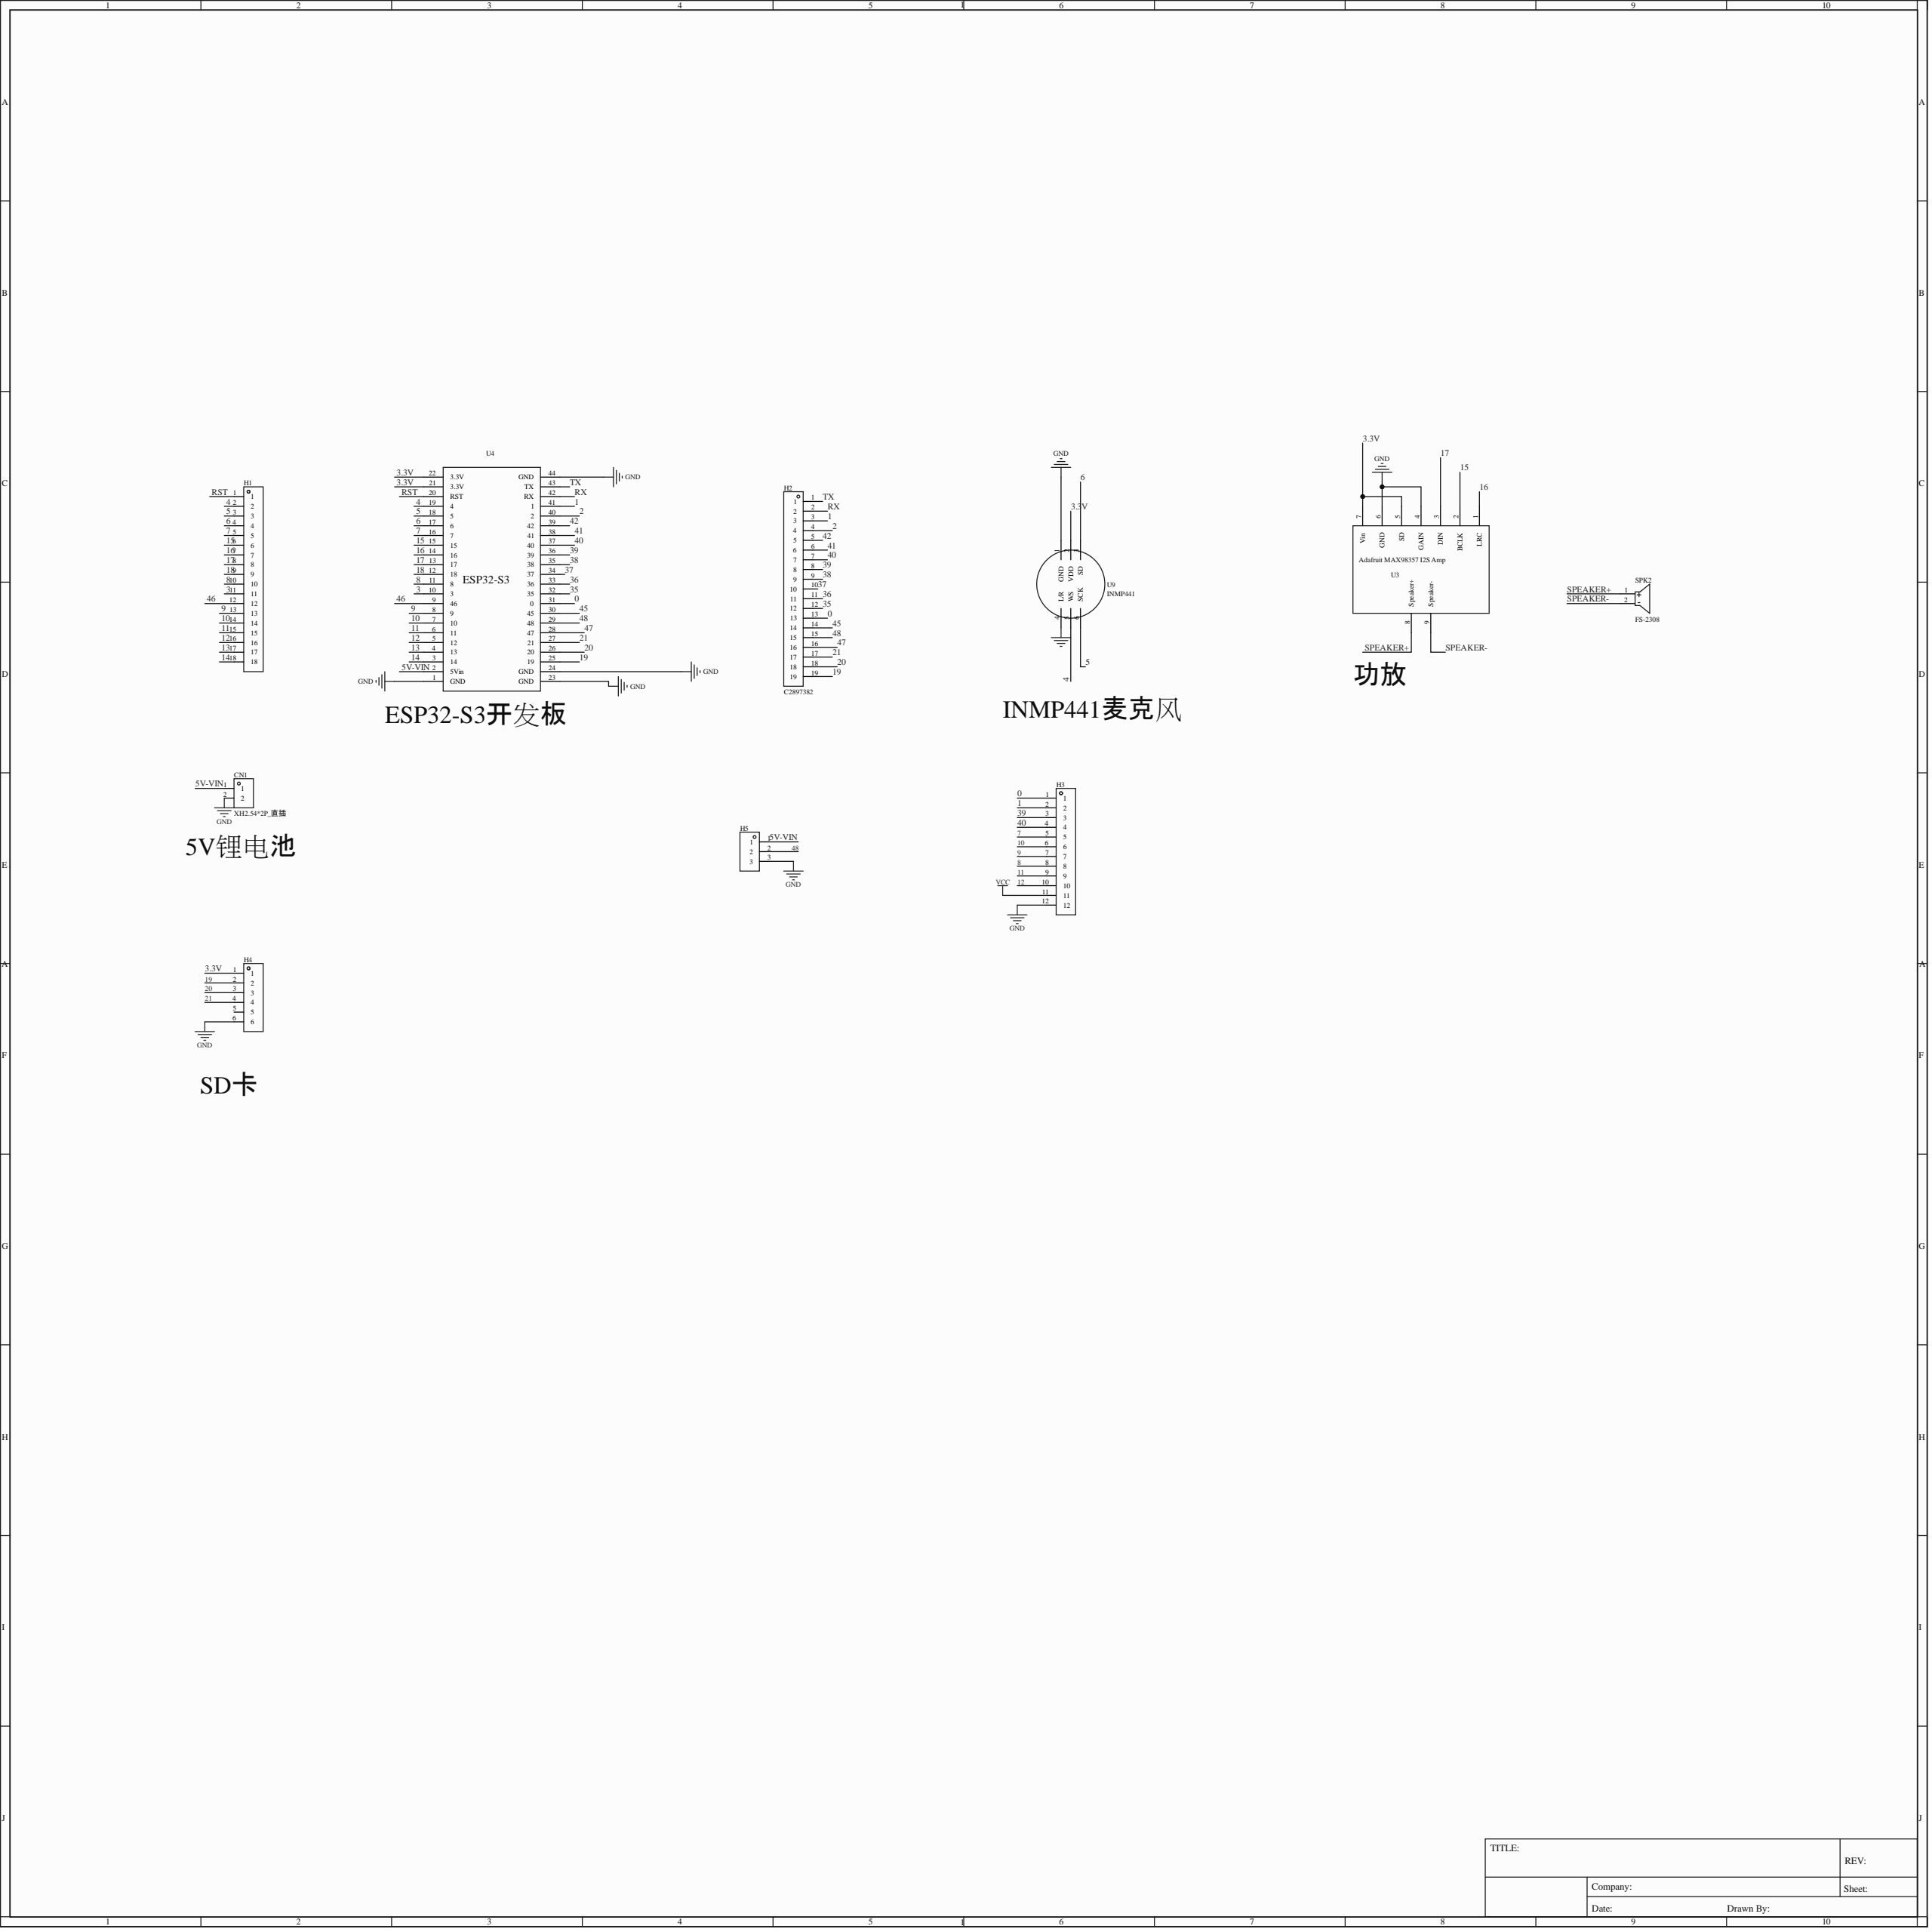Circuit board | Altium Designer | 10 parts | 42 nets
Bill of materials:
Comment,Description,Designator,Footprint,LibRef,Quantity
"XH2.54*2P_直插","","CN1","CONN-TH_2P-P2.50-XH2.54-2P","XH2.54*2P_直插","1"
"","","H1","HDR-TH_18P-P2.54-V-F","HDR-F_2.54_1x18P","1"
"C2897382","","H2","HDR-TH_19P-P2.54-V-F","HDR-F_2.54_1x19P","1"
"","","H3","HDR-TH_12P-P2.54-V-F","HDR-F_2.54_1x12P","1"
"","","H4","HDR-TH_6P-P2.54-V-F","HDR-F_2.54_1x6P","1"
"","","H5","HDR-TH_3P-P2.54-V-F","HDR-F_2.54_1x3P","1"
"FS-2308","","SPK2","BEEP-TH_BD23.2-P9.20-D1.0","FS-2308","1"
"Adafruit MAX98357 I2S Amp","","U3","MAX98357 I2S AMP MODULE","Adafruit MAX98357 I2S Amp","1"
"NO","","U4","ESP32S3","NO","1"
"INMP441","","U9","INMP441","INMP441","1"
Netlist (Protel format):
[
CN1
CONN-TH_2P-P2.50-XH2.54-2P
XH2.54*2P_直插



]
[
H1
HDR-TH_18P-P2.54-V-F




]
[
H2
HDR-TH_19P-P2.54-V-F
C2897382



]
[
H3
HDR-TH_12P-P2.54-V-F




]
[
H4
HDR-TH_6P-P2.54-V-F




]
[
H5
HDR-TH_3P-P2.54-V-F




]
[
SPK2
BEEP-TH_BD23.2-P9.20-D1.0
FS-2308



]
[
U3
MAX98357 I2S AMP MODULE
Adafruit MAX98357 I2S Amp



]
[
U4
ESP32S3
NO



]
[
U9
INMP441
INMP441



]
(
TX
H2-1
U4-43
)
(
SPEAKER-
SPK2-2
U3-9
)
(
SPEAKER+
SPK2-1
U3-8
)
(
RX
H2-2
U4-42
)
(
RST
H1-1
U4-20
)
(
GND
CN1-2
H3-12
H4-6
H5-3
U3-4
U3-6
U4-1
U4-23
U4-24
U4-44
U9-1
U9-4
)
(
48
H2-15
H5-2
U4-29
)
(
47
H2-16
U4-28
)
(
46
H1-12
U4-9
)
(
45
H2-14
U4-30
)
(
42
H2-5
U4-39
)
(
41
H2-6
U4-38
)
(
40
H2-7
H3-4
U4-37
)
(
39
H2-8
H3-3
U4-36
)
(
38
H2-9
U4-35
)
(
37
H2-10
U4-34
)
(
36
H2-11
U4-33
)
(
35
H2-12
U4-32
)
(
21
H2-17
H4-4
U4-27
)
(
20
H2-18
H4-3
U4-26
)
(
19
H2-19
H4-2
U4-25
)
(
18
H1-9
U4-12
)
(
17
H1-8
U3-3
U4-13
)
(
16
H1-7
U3-1
U4-14
)
(
15
H1-6
U3-2
U4-15
)
(
14
H1-18
U4-3
)
(
13
H1-17
U4-4
)
(
12
H1-16
H3-10
U4-5
)
(
11
H1-15
H3-9
U4-6
)
(
10
H1-14
H3-6
U4-7
)
(
9
H1-13
H3-7
U4-8
)
(
8
H1-10
H3-8
U4-11
)
(
7
H1-5
H3-5
U4-16
)
(
6
H1-4
U4-17
U9-3
)
(
5V-VIN
CN1-1
H5-1
U4-2
)
(
5
H1-3
U4-18
U9-6
)
(
4
H1-2
U4-19
U9-5
)
(
3.3V
H4-1
U3-5
U3-7
U4-21
U4-22
U9-2
)
(
3
H1-11
U4-10
)
(
2
H2-4
U4-40
)
(
1
H2-3
H3-2
U4-41
)
(
0
H2-13
H3-1
U4-31
)